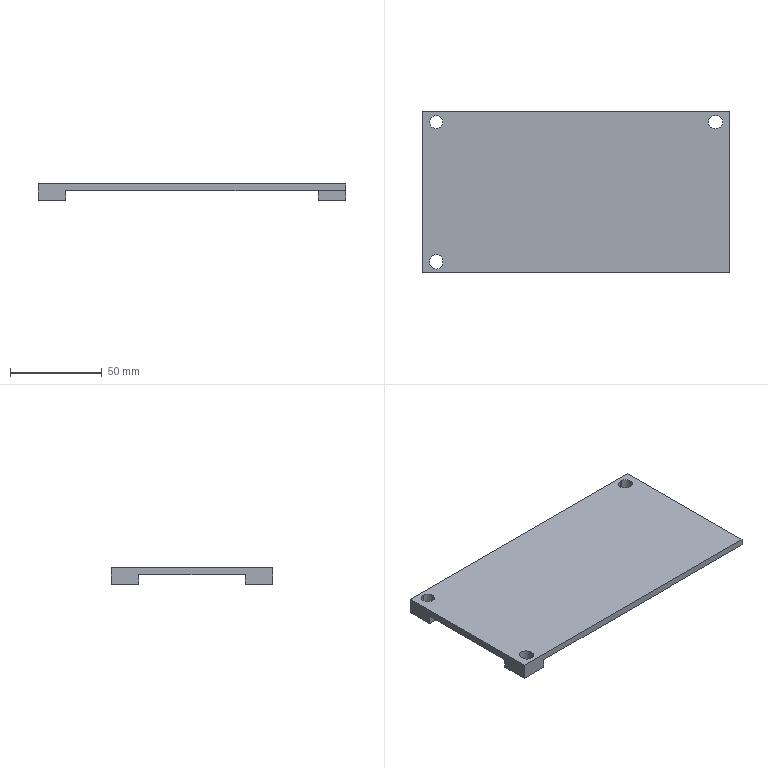NC program | NX | posted with a generic post | part box 168 x 88.2 x 8.8 mm
Whole program:
N10 G17 G21 G94 G90
(FLOOR_WALL_COPY , TOOL : D80)
N12 T19 M6
N14 G54
N16 G17 G0 G90 X127. Y-44.097 S5000 M3
N18 G43 Z30. H19
N20 Z7.
N22 G94 G1 Z4. F1200.
N24 X124.
N26 X-124.
N28 Y-33.364
N30 Y-15.999
N32 X124.
N34 Y12.1
N36 X-124.
N38 X-127.
N40 Z7.
N42 G0 Z30.
N44 X127. Y-44.097
N46 Z6.
N48 G1 Z3.
N50 X124.
N52 X-124.
N54 Y-33.364
N56 Y-15.999
N58 X124.
N60 Y12.1
N62 X-124.
N64 X-127.
N66 Z6.
N68 G0 Z30.
N70 X127. Y-44.097
N72 Z5.
N74 G1 Z2.
N76 X124.
N78 X-124.
N80 Y-33.364
N82 Y-15.999
N84 X124.
N86 Y12.1
N88 X-124.
N90 X-127.
N92 Z5.
N94 G0 Z30.
N96 X127. Y-44.097
N98 Z4.
N100 G1 Z1.
N102 X124.
N104 X-124.
N106 Y-33.364
N108 Y-15.999
N110 X124.
N112 Y12.1
N114 X-124.
N116 X-127.
N118 Z4.
N120 G0 Z30.
N122 X127. Y-44.097
N124 Z3.
N126 G1 Z0.
N128 X124.
N130 X-124.
N132 Y-15.999
N134 X124.
N136 Y12.1
N138 X-124.
N140 X-127.
N142 Z3.
N144 G0 Z30.
N146 M5
(FLOOR_WALL_1 , TOOL : D10)
N148 T15 M6
N150 G54
N152 G17 G0 G90 X-0.808 Y50.6 S9500 M3
N154 G43 Z30. H15
N156 Z0.52
N158 G94 G1 Z-0.98 F1000.
N160 X-0.231 Y49.6
N162 G3 X0.635 Y49.1 R1.
N164 G1 X89. F3000.
N166 Y-24.
N168 X63.9
N170 Y-49.1
N172 X-63.9
N174 Y-43.1
N176 Y-24.
N178 X-89.
N180 Y24.
N182 X-83.
N184 X-63.9
N186 Y49.1
N188 X0.635
N190 Y43.1
N192 X83.
N194 Y-18.
N196 X63.9
N198 G3 X57.9 Y-24. R6.
N200 G1 Y-43.1
N202 X-57.9
N204 Y-24.
N206 G3 X-62.748 Y-18.112 R6.
N208 G1 X-63.319 Y-18.
N210 X-83.
N212 Y18.
N214 X-63.9
N216 G3 X-57.9 Y24. R6.
N218 G1 Y43.1
N220 X0.635
N222 Y37.1
N224 X77.
N226 Y-12.
N228 X63.9
N230 G3 X51.9 Y-24. R12.
N232 G1 Y-37.1
N234 X-51.9
N236 Y-24.
N238 G3 X-61.597 Y-12.223 R12.
N240 G1 X-62.737 Y-12.
N242 X-77.
N244 Y12.
N246 X-63.9
N248 G3 X-51.9 Y24. R12.
N250 G1 Y37.1
N252 X0.635
N254 Y31.1
N256 X71.
N258 Y-6.
N260 X63.9
N262 G3 X45.9 Y-24. R18.
N264 G1 Y-31.1
N266 X-45.9
N268 Y-24.
N270 G3 X-60.445 Y-6.335 R18.
N272 G1 X-62.156 Y-6.
N274 X-71.
N276 Y6.
N278 X-63.9
N280 G3 X-45.9 Y24. R18.
N282 G1 Y31.1
N284 X0.635
N286 Y25.1
N288 X65.
N290 Y0.
N292 X63.9
N294 G3 X39.9 Y-24. R24.
N296 G1 Y-25.1
N298 X-39.9
N300 Y-24.
N302 G3 X-59.293 Y-0.446 R24.
N304 G1 X-61.575 Y0.
N306 X-65.
N308 X-63.9
N310 G3 X-39.9 Y24. R24.
N312 G1 Y25.1
N314 X0.635
N316 Y19.1
N318 X59.
N320 Y5.597
N322 G3 X34.303 Y-19.1 R30.
N324 G1 X-34.303
N326 G3 X-45.9 Y0. R30.
N328 X-34.303 Y19.1 R30.
N330 G1 X0.635
N332 Y13.1
N334 X53.
N336 Y10.31
N338 G3 X29.59 Y-13.1 R36.
N340 G1 X-29.59
N342 G3 X-37.067 Y0. R36.
N344 X-29.59 Y13.1 R36.
N346 G1 X0.635
N348 Y7.1
N350 X35.673
N352 G3 X25.45 Y-7.1 R42.
N354 G1 X-25.45
N356 G3 X-29.433 Y0. R42.
N358 X-25.45 Y7.1 R42.
N360 G1 X0.635
N362 Y1.1
N364 X22.986
N366 G3 X21.715 Y-1.1 R48.
N368 G1 X-21.715
N370 G3 X-22.331 Y0. R48.
N372 X-21.715 Y1.1 R48.
N374 G1 X0.635
N376 G3 X1.501 Y1.6 R1.
N378 G1 Z0.52
N380 G0 X-0.808 Y50.6 Z-0.46
N382 G1 Z-1.96 F1000.
N384 X-0.231 Y49.6
N386 G3 X0.635 Y49.1 R1.
N388 G1 X89. F3000.
N390 Y-24.
N392 X63.9
N394 Y-49.1
N396 X-63.9
N398 Y-43.1
N400 Y-24.
N402 X-89.
N404 Y24.
N406 X-83.
N408 X-63.9
N410 Y49.1
N412 X0.635
N414 Y43.1
N416 X83.
N418 Y-18.
N420 X63.9
N422 G3 X57.9 Y-24. R6.
N424 G1 Y-43.1
N426 X-57.9
N428 Y-24.
N430 G3 X-62.748 Y-18.112 R6.
N432 G1 X-63.319 Y-18.
N434 X-83.
N436 Y18.
N438 X-63.9
N440 G3 X-57.9 Y24. R6.
N442 G1 Y43.1
N444 X0.635
N446 Y37.1
N448 X77.
N450 Y-12.
N452 X63.9
N454 G3 X51.9 Y-24. R12.
N456 G1 Y-37.1
N458 X-51.9
N460 Y-24.
N462 G3 X-61.597 Y-12.223 R12.
N464 G1 X-62.737 Y-12.
N466 X-77.
N468 Y12.
N470 X-63.9
N472 G3 X-51.9 Y24. R12.
N474 G1 Y37.1
N476 X0.635
N478 Y31.1
N480 X71.
N482 Y-6.
N484 X63.9
N486 G3 X45.9 Y-24. R18.
N488 G1 Y-31.1
N490 X-45.9
N492 Y-24.
N494 G3 X-60.445 Y-6.335 R18.
N496 G1 X-62.156 Y-6.
N498 X-71.
N500 Y6.
N502 X-63.9
N504 G3 X-45.9 Y24. R18.
N506 G1 Y31.1
N508 X0.635
N510 Y25.1
N512 X65.
N514 Y0.
N516 X63.9
N518 G3 X39.9 Y-24. R24.
N520 G1 Y-25.1
N522 X-39.9
N524 Y-24.
N526 G3 X-59.293 Y-0.446 R24.
N528 G1 X-61.575 Y0.
N530 X-65.
N532 X-63.9
N534 G3 X-39.9 Y24. R24.
N536 G1 Y25.1
N538 X0.635
N540 Y19.1
N542 X59.
N544 Y5.597
N546 G3 X34.303 Y-19.1 R30.
N548 G1 X-34.303
N550 G3 X-45.9 Y0. R30.
N552 X-34.303 Y19.1 R30.
N554 G1 X0.635
N556 Y13.1
N558 X53.
N560 Y10.31
N562 G3 X29.59 Y-13.1 R36.
N564 G1 X-29.59
N566 G3 X-37.067 Y0. R36.
N568 X-29.59 Y13.1 R36.
N570 G1 X0.635
N572 Y7.1
N574 X35.673
N576 G3 X25.45 Y-7.1 R42.
N578 G1 X-25.45
N580 G3 X-29.433 Y0. R42.
N582 X-25.45 Y7.1 R42.
N584 G1 X0.635
N586 Y1.1
N588 X22.986
N590 G3 X21.715 Y-1.1 R48.
N592 G1 X-21.715
N594 G3 X-22.331 Y0. R48.
N596 X-21.715 Y1.1 R48.
N598 G1 X0.635
N600 G3 X1.501 Y1.6 R1.
N602 G1 Z-0.46
N604 G0 X-0.808 Y50.6 Z-1.44
N606 G1 Z-2.94 F1000.
N608 X-0.231 Y49.6
N610 G3 X0.635 Y49.1 R1.
N612 G1 X89. F3000.
N614 Y-24.
N616 X63.9
N618 Y-49.1
N620 X-63.9
N622 Y-43.1
N624 Y-24.
N626 X-89.
N628 Y24.
N630 X-83.
N632 X-63.9
N634 Y49.1
N636 X0.635
N638 Y43.1
N640 X83.
N642 Y-18.
N644 X63.9
N646 G3 X57.9 Y-24. R6.
N648 G1 Y-43.1
N650 X-57.9
N652 Y-24.
N654 G3 X-62.748 Y-18.112 R6.
N656 G1 X-63.319 Y-18.
N658 X-83.
N660 Y18.
N662 X-63.9
N664 G3 X-57.9 Y24. R6.
N666 G1 Y43.1
N668 X0.635
N670 Y37.1
N672 X77.
N674 Y-12.
N676 X63.9
N678 G3 X51.9 Y-24. R12.
N680 G1 Y-37.1
N682 X-51.9
N684 Y-24.
N686 G3 X-61.597 Y-12.223 R12.
N688 G1 X-62.737 Y-12.
N690 X-77.
N692 Y12.
N694 X-63.9
N696 G3 X-51.9 Y24. R12.
N698 G1 Y37.1
N700 X0.635
N702 Y31.1
N704 X71.
N706 Y-6.
N708 X63.9
N710 G3 X45.9 Y-24. R18.
N712 G1 Y-31.1
N714 X-45.9
N716 Y-24.
N718 G3 X-60.445 Y-6.335 R18.
N720 G1 X-62.156 Y-6.
N722 X-71.
N724 Y6.
N726 X-63.9
N728 G3 X-45.9 Y24. R18.
N730 G1 Y31.1
N732 X0.635
N734 Y25.1
N736 X65.
N738 Y0.
N740 X63.9
N742 G3 X39.9 Y-24. R24.
N744 G1 Y-25.1
N746 X-39.9
N748 Y-24.
N750 G3 X-59.293 Y-0.446 R24.
N752 G1 X-61.575 Y0.
N754 X-65.
N756 X-63.9
N758 G3 X-39.9 Y24. R24.
N760 G1 Y25.1
N762 X0.635
N764 Y19.1
N766 X59.
N768 Y5.597
N770 G3 X34.303 Y-19.1 R30.
N772 G1 X-34.303
N774 G3 X-45.9 Y0. R30.
N776 X-34.303 Y19.1 R30.
N778 G1 X0.635
N780 Y13.1
N782 X53.
N784 Y10.31
N786 G3 X29.59 Y-13.1 R36.
N788 G1 X-29.59
N790 G3 X-37.067 Y0. R36.
N792 X-29.59 Y13.1 R36.
N794 G1 X0.635
N796 Y7.1
N798 X35.673
N800 G3 X25.45 Y-7.1 R42.
N802 G1 X-25.45
N804 G3 X-29.433 Y0. R42.
N806 X-25.45 Y7.1 R42.
N808 G1 X0.635
N810 Y1.1
N812 X22.986
N814 G3 X21.715 Y-1.1 R48.
N816 G1 X-21.715
N818 G3 X-22.331 Y0. R48.
N820 X-21.715 Y1.1 R48.
N822 G1 X0.635
N824 G3 X1.501 Y1.6 R1.
N826 G1 Z-1.44
N828 G0 X-0.808 Y50.6 Z-2.42
N830 G1 Z-3.92 F1000.
N832 X-0.231 Y49.6
N834 G3 X0.635 Y49.1 R1.
N836 G1 X89. F3000.
N838 Y-24.
N840 X63.9
N842 Y-49.1
N844 X-63.9
N846 Y-43.1
N848 Y-24.
N850 X-89.
N852 Y24.
N854 X-83.
N856 X-63.9
N858 Y49.1
N860 X0.635
N862 Y43.1
N864 X83.
N866 Y-18.
N868 X63.9
N870 G3 X57.9 Y-24. R6.
N872 G1 Y-43.1
N874 X-57.9
N876 Y-24.
N878 G3 X-62.748 Y-18.112 R6.
N880 G1 X-63.319 Y-18.
N882 X-83.
N884 Y18.
N886 X-63.9
N888 G3 X-57.9 Y24. R6.
N890 G1 Y43.1
N892 X0.635
N894 Y37.1
N896 X77.
N898 Y-12.
N900 X63.9
N902 G3 X51.9 Y-24. R12.
N904 G1 Y-37.1
N906 X-51.9
N908 Y-24.
N910 G3 X-61.597 Y-12.223 R12.
N912 G1 X-62.737 Y-12.
N914 X-77.
N916 Y12.
N918 X-63.9
N920 G3 X-51.9 Y24. R12.
N922 G1 Y37.1
N924 X0.635
N926 Y31.1
N928 X71.
N930 Y-6.
N932 X63.9
N934 G3 X45.9 Y-24. R18.
N936 G1 Y-31.1
N938 X-45.9
N940 Y-24.
N942 G3 X-60.445 Y-6.335 R18.
N944 G1 X-62.156 Y-6.
N946 X-71.
N948 Y6.
N950 X-63.9
N952 G3 X-45.9 Y24. R18.
N954 G1 Y31.1
N956 X0.635
N958 Y25.1
N960 X65.
N962 Y0.
N964 X63.9
N966 G3 X39.9 Y-24. R24.
N968 G1 Y-25.1
N970 X-39.9
N972 Y-24.
N974 G3 X-59.293 Y-0.446 R24.
N976 G1 X-61.575 Y0.
N978 X-65.
N980 X-63.9
N982 G3 X-39.9 Y24. R24.
N984 G1 Y25.1
N986 X0.635
N988 Y19.1
N990 X59.
N992 Y5.597
N994 G3 X34.303 Y-19.1 R30.
N996 G1 X-34.303
N998 G3 X-45.9 Y0. R30.
N1000 X-34.303 Y19.1 R30.
N1002 G1 X0.635
N1004 Y13.1
N1006 X53.
N1008 Y10.31
N1010 G3 X29.59 Y-13.1 R36.
N1012 G1 X-29.59
N1014 G3 X-37.067 Y0. R36.
N1016 X-29.59 Y13.1 R36.
N1018 G1 X0.635
N1020 Y7.1
N1022 X35.673
N1024 G3 X25.45 Y-7.1 R42.
N1026 G1 X-25.45
N1028 G3 X-29.433 Y0. R42.
N1030 X-25.45 Y7.1 R42.
N1032 G1 X0.635
N1034 Y1.1
N1036 X22.986
N1038 G3 X21.715 Y-1.1 R48.
N1040 G1 X-21.715
N1042 G3 X-22.331 Y0. R48.
N1044 X-21.715 Y1.1 R48.
N1046 G1 X0.635
N1048 G3 X1.501 Y1.6 R1.
N1050 G1 Z-2.42
N1052 G0 X-0.808 Y50.6 Z-3.4
N1054 G1 Z-4.9 F1000.
N1056 X-0.231 Y49.6
N1058 G3 X0.635 Y49.1 R1.
N1060 G1 X89. F3000.
N1062 Y-24.
N1064 X63.9
N1066 Y-49.1
N1068 X-63.9
N1070 Y-43.1
N1072 Y-24.
N1074 X-89.
N1076 Y24.
N1078 X-83.
N1080 X-63.9
N1082 Y49.1
N1084 X0.635
N1086 Y43.1
N1088 X83.
N1090 Y-18.
N1092 X63.9
N1094 G3 X57.9 Y-24. R6.
N1096 G1 Y-43.1
N1098 X-57.9
N1100 Y-24.
N1102 G3 X-62.748 Y-18.112 R6.
N1104 G1 X-63.319 Y-18.
N1106 X-83.
N1108 Y18.
N1110 X-63.9
N1112 G3 X-57.9 Y24. R6.
N1114 G1 Y43.1
N1116 X0.635
N1118 Y37.1
N1120 X77.
N1122 Y-12.
N1124 X63.9
N1126 G3 X51.9 Y-24. R12.
N1128 G1 Y-37.1
N1130 X-51.9
N1132 Y-24.
N1134 G3 X-61.597 Y-12.223 R12.
N1136 G1 X-62.737 Y-12.
N1138 X-77.
N1140 Y12.
N1142 X-63.9
N1144 G3 X-51.9 Y24. R12.
N1146 G1 Y37.1
N1148 X0.635
N1150 Y31.1
N1152 X71.
N1154 Y-6.
N1156 X63.9
N1158 G3 X45.9 Y-24. R18.
N1160 G1 Y-31.1
N1162 X-45.9
N1164 Y-24.
N1166 G3 X-60.445 Y-6.335 R18.
N1168 G1 X-62.156 Y-6.
N1170 X-71.
N1172 Y6.
N1174 X-63.9
N1176 G3 X-45.9 Y24. R18.
N1178 G1 Y31.1
N1180 X0.635
N1182 Y25.1
N1184 X65.
N1186 Y0.
N1188 X63.9
N1190 G3 X39.9 Y-24. R24.
N1192 G1 Y-25.1
N1194 X-39.9
N1196 Y-24.
N1198 G3 X-59.293 Y-0.446 R24.
N1200 G1 X-61.575 Y0.
N1202 X-65.
N1204 X-63.9
N1206 G3 X-39.9 Y24. R24.
N1208 G1 Y25.1
N1210 X0.635
N1212 Y19.1
N1214 X59.
N1216 Y5.597
N1218 G3 X34.303 Y-19.1 R30.
N1220 G1 X-34.303
N1222 G3 X-45.9 Y0. R30.
N1224 X-34.303 Y19.1 R30.
N1226 G1 X0.635
N1228 Y13.1
N1230 X53.
N1232 Y10.31
N1234 G3 X29.59 Y-13.1 R36.
N1236 G1 X-29.59
N1238 G3 X-37.067 Y0. R36.
N1240 X-29.59 Y13.1 R36.
N1242 G1 X0.635
N1244 Y7.1
N1246 X35.673
N1248 G3 X25.45 Y-7.1 R42.
N1250 G1 X-25.45
N1252 G3 X-29.433 Y0. R42.
N1254 X-25.45 Y7.1 R42.
N1256 G1 X0.635
N1258 Y1.1
N1260 X22.986
N1262 G3 X21.715 Y-1.1 R48.
N1264 G1 X-21.715
N1266 G3 X-22.331 Y0. R48.
N1268 X-21.715 Y1.1 R48.
N1270 G1 X0.635
N1272 G3 X1.501 Y1.6 R1.
N1274 G1 Z-3.4
N1276 G0 Z30.
N1278 M5
(FLOOR_WALL_1_COPY , TOOL : D10JING)
N1280 T14 M6
N1282 G54
N1284 G17 G0 G90 X89.975 Y-3.727 S9500 M3
N1286 G43 Z30. H14
N1288 Z-3.5
N1290 G94 G1 Z-5. F1000.
N1292 X89.5 Y-4.001
N1294 G3 X89. Y-4.867 R1.
N1296 G1 Y-23.6 F1400.
N1298 X83.172
N1300 Y-4.867
N1302 X77.345
N1304 Y-23.6
N1306 X71.517
N1308 Y-4.867
N1310 X65.69
N1312 Y-23.6
N1314 X64.
N1316 G3 X63.5 Y-24.1 R0.5
N1318 G1 Y-49.1
N1320 X59.862
N1322 Y-4.867
N1324 X54.034
N1326 Y-49.1
N1328 X48.207
N1330 Y-4.867
N1332 X42.379
N1334 Y-49.1
N1336 X36.552
N1338 Y-4.867
N1340 X33.934 Y49.1
N1342 X30.724
N1344 Y-49.1
N1346 X24.897
N1348 Y49.1
N1350 X19.069
N1352 Y-49.1
N1354 X13.241
N1356 Y49.1
N1358 X7.414
N1360 Y-49.1
N1362 X1.586
N1364 Y49.1
N1366 X-4.241
N1368 Y-49.1
N1370 X-10.069
N1372 Y49.1
N1374 X-15.897
N1376 Y-49.1
N1378 X-21.724
N1380 Y49.1
N1382 X-27.552
N1384 Y-49.1
N1386 X-33.379
N1388 Y49.1
N1390 X-39.207
N1392 Y-49.1
N1394 X-45.034
N1396 Y49.1
N1398 X-50.862
N1400 Y-49.1
N1402 X-56.69
N1404 Y49.1
N1406 X-62.517
N1408 Y-49.1
N1410 X-63.5
N1412 Y-24.1
N1414 G3 X-64. Y-23.6 R0.5
N1416 G1 X-68.345
N1418 Y23.6
N1420 X-74.172
N1422 Y-23.6
N1424 X-80.
N1426 Y23.6
N1428 Z-3.5
N1430 G0 Z30.
N1432 X-62.402 Y50.6
N1434 Z-3.5
N1436 G1 Z-5. F1000.
N1438 X-63.5 Y49.966
N1440 G3 X-64. Y49.1 R1.
N1442 G1 Y24.1 F1400.
N1444 X-89.
N1446 G3 X-89.866 Y23.6 R1.
N1448 G1 X-90.5 Y22.502
N1450 Z-3.5
N1452 G0 Z-1.9
N1454 Y-22.502
N1456 Z-3.5
N1458 G1 Z-5. F1000.
N1460 X-89.866 Y-23.6
N1462 G3 X-89. Y-24.1 R1.
N1464 G1 X-64. F1400.
N1466 Y-49.1
N1468 G3 X-63.5 Y-49.966 R1.
N1470 G1 X-62.402 Y-50.6
N1472 Z-3.5
N1474 G0 Z-1.9
N1476 X62.402
N1478 Z-3.5
N1480 G1 Z-5. F1000.
N1482 X63.5 Y-49.966
N1484 G3 X64. Y-49.1 R1.
N1486 G1 Y-24.1 F1400.
N1488 X89.
N1490 G3 X89.866 Y-23.6 R1.
N1492 G1 X90.5 Y-22.502
N1494 Z-3.5
N1496 G0 Z30.
N1498 Y-3.864
N1500 Z-3.7
N1502 G1 Z-5.2 F1000.
N1504 X88.134
N1506 G3 X89. Y-4.364 R1.
N1508 G1 X34.434 F1400.
N1510 Y1.194
N1512 X89.
N1514 Y6.752
N1516 X34.434
N1518 Y12.31
N1520 X89.
N1522 Y17.868
N1524 X34.434
N1526 Y23.426
N1528 X89.
N1530 Y28.984
N1532 X34.434
N1534 Y34.542
N1536 X89.
N1538 Y40.1
N1540 X34.434
N1542 G3 X34.934 Y39.234 R1.
N1544 G1 Z-3.7
N1546 G0 Z-2.1
N1548 X35.532 Y50.6
N1550 Z-3.7
N1552 G1 Z-5.2 F1000.
N1554 X34.434 Y49.966
N1556 G3 X33.934 Y49.1 R1.
N1558 G1 Y-4.867 F1400.
N1560 X89.
N1562 G3 X89.866 Y-4.367 R1.
N1564 G1 X90.5 Y-3.269
N1566 Z-3.7
N1568 G0 Z30.
N1570 M5
(ZLEVEL_PROFILE_COPY_1 , TOOL : D4)
N1572 T11 M6
N1574 G54
N1576 G17 G0 G90 X32.934 Y-3.328 S9500 M3
N1578 G43 Z30. H11
N1580 Z-2.2
N1582 G94 G1 Z-5.2 F1000.
N1584 X31.134 Y-4.368
N1586 G3 X30.934 Y-4.714 R0.4
N1588 G1 Y-7.867 F1500.
N1590 X34.087
N1592 G3 X34.433 Y-7.667 R0.4
N1594 G1 X35.473 Y-5.867
N1596 Z-2.2
N1598 G0 Z30.
N1600 M5
(PLANAR_PROFILE_COPY , TOOL : D6A45)
N1602 T01 M6
N1604 G54
N1606 G17 G0 G90 X68.278 Y-27.377 S9500 M3
N1608 G43 Z30. H1
N1610 Z0.5
N1612 G94 G1 Z-1. F1500.
N1614 X68.58 Y-27.9
N1616 G3 X69.1 Y-28.2 R0.6
N1618 G1 X83.9
N1620 G2 X84.9 Y-29.2 R1.
N1622 G1 Y-44.
N1624 G2 X83.9 Y-45. R1.
N1626 G1 X69.1
N1628 G2 X68.1 Y-44. R1.
N1630 G1 Y-29.2
N1632 G2 X69.1 Y-28.2 R1.
N1634 G3 X69.62 Y-27.9 R0.6
N1636 G1 X70.024 Y-27.2
N1638 Z0.5
N1640 G0 Z30.
N1642 X75.69 Y-39.782
N1644 Z0.5
N1646 G1 Z-1.
N1648 X76.095 Y-40.485
N1650 G3 X76.615 Y-40.785 R0.6
N1652 X79.3 Y-38.1 R2.685
N1654 X76.615 Y-35.415 R2.685
N1656 G1 X75.785
N1658 G3 X73.1 Y-38.1 R2.685
N1660 X75.785 Y-40.785 R2.685
N1662 G1 X76.615
N1664 G3 X77.135 Y-40.485 R0.6
N1666 G1 X77.849 Y-39.247
N1668 Z0.5
N1670 G0 Z30.
N1672 X-74.966 Y-36.953
N1674 Z0.5
N1676 G1 Z-1.
N1678 X-75.68 Y-35.715
N1680 G3 X-76.2 Y-35.415 R0.6
N1682 X-78.885 Y-38.1 R2.685
N1684 X-76.2 Y-35.415 R-2.685
N1686 X-76.72 Y-35.715 R0.6
N1688 G1 X-77.434 Y-36.953
N1690 Z0.5
N1692 G0 Z30.
N1694 X-67.277 Y-28.378
N1696 Z0.5
N1698 G1 Z-1.
N1700 X-67.8 Y-28.68
N1702 G3 X-68.1 Y-29.2 R0.6
N1704 G1 Y-44.
N1706 G2 X-69.1 Y-45. R1.
N1708 G1 X-83.9
N1710 G2 X-84.9 Y-44. R1.
N1712 G1 Y-29.2
N1714 G2 X-83.9 Y-28.2 R1.
N1716 G1 X-69.1
N1718 G2 X-68.1 Y-29.2 R1.
N1720 G3 X-67.8 Y-29.72 R0.6
N1722 G1 X-67.1 Y-30.124
N1724 Z0.5
N1726 G0 Z30.
N1728 X-68.278 Y27.377
N1730 Z0.5
N1732 G1 Z-1.
N1734 X-68.58 Y27.9
N1736 G3 X-69.1 Y28.2 R0.6
N1738 G1 X-83.9
N1740 G2 X-84.9 Y29.2 R1.
N1742 G1 Y44.
N1744 G2 X-83.9 Y45. R1.
N1746 G1 X-69.1
N1748 G2 X-68.1 Y44. R1.
N1750 G1 Y29.2
N1752 G2 X-69.1 Y28.2 R1.
N1754 G3 X-69.62 Y27.9 R0.6
N1756 G1 X-70.024 Y27.2
N1758 Z0.5
N1760 G0 Z30.
N1762 X-77.434 Y36.538
N1764 Z0.5
N1766 G1 Z-1.
N1768 X-76.72 Y35.3
N1770 G3 X-76.2 Y35. R0.6
N1772 X-73.515 Y37.685 R2.685
N1774 G1 Y38.515
N1776 G3 X-76.2 Y41.2 R2.685
N1778 X-78.885 Y38.515 R2.685
N1780 G1 Y37.685
N1782 G3 X-76.2 Y35. R2.685
N1784 X-75.68 Y35.3 R0.6
N1786 G1 X-74.966 Y36.538
N1788 Z0.5
N1790 G0 Z30.
(PLANAR_PROFILE_COPY_COPY , TOOL : D6A45)
N1792 X85.9 Y-8.943
N1794 Z-4.5
N1796 G1 Z-6.
N1798 X85.2 Y-9.347
N1800 G3 X84.9 Y-9.867 R0.6
N1802 G1 Y-25.718
N1804 G3 X85.479 Y-25.561 R0.6
N1806 G1 X85.98 Y-25.059
N1808 Z-4.5
N1810 G0 Z30.
N1812 X64.959 Y-46.08
N1814 Z-4.5
N1816 G1 Z-6.
N1818 X65.461 Y-45.579
N1820 G3 X65.618 Y-45. R0.6
N1822 G1 X-65.618
N1824 G3 X-65.461 Y-45.579 R0.6
N1826 G1 X-64.959 Y-46.08
N1828 Z-4.5
N1830 G0 Z30.
N1832 X-85.98 Y-25.059
N1834 Z-4.5
N1836 G1 Z-6.
N1838 X-85.479 Y-25.561
N1840 G3 X-84.9 Y-25.718 R0.6
N1842 G1 Y25.718
N1844 G3 X-85.479 Y25.561 R0.6
N1846 G1 X-85.98 Y25.059
N1848 Z-4.5
N1850 G0 Z30.
N1852 X-64.959 Y46.08
N1854 Z-4.5
N1856 G1 Z-6.
N1858 X-65.461 Y45.579
N1860 G3 X-65.618 Y45. R0.6
N1862 G1 X28.934
N1864 G3 X29.454 Y45.3 R0.6
N1866 G1 X29.858 Y46.
N1868 Z-4.5
N1870 G0 Z30.
(PLANAR_PROFILE_COPY_COPY_COPY , TOOL : D6A45)
N1872 X28.01
N1874 Z-4.7
N1876 G1 Z-6.2
N1878 X28.414 Y45.3
N1880 G3 X28.934 Y45. R0.6
N1882 G1 X83.9
N1884 G2 X84.9 Y44. R1.
N1886 G1 Y-9.867
N1888 G3 X85.2 Y-10.387 R0.6
N1890 G1 X85.9 Y-10.791
N1892 Z-4.7
N1894 G0 Z30.
N1896 M5
N1898 M2